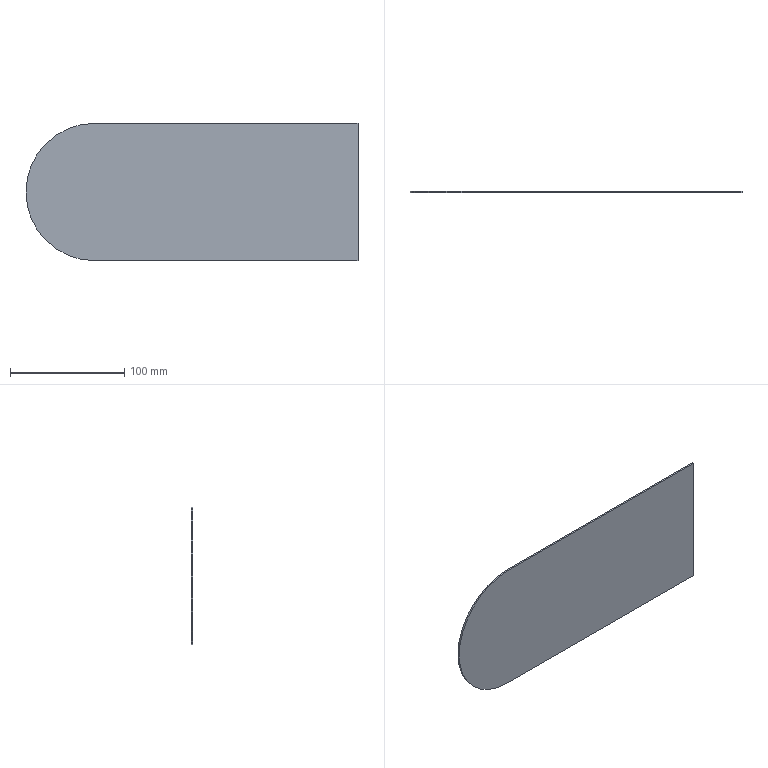Part | SolidWorks | features BaseBody 1 | 1 solid | 6 faces | box 290 x 1.5 x 120 mm | volume 49882 mm3 | plane 5 | cylinder 1 | commonest cylinder face diameters 120 x1
STEP:
#1=CARTESIAN_POINT('',(-115.,-1.5,60.));
#2=VERTEX_POINT('',#1);
#3=CARTESIAN_POINT('',(115.,-1.5,60.));
#4=VERTEX_POINT('',#3);
#5=CARTESIAN_POINT('',(-115.,-1.5,60.));
#6=DIRECTION('',(1.,0.,0.));
#7=VECTOR('',#6,1000.);
#8=LINE('',#5,#7);
#9=EDGE_CURVE('',#2,#4,#8,.T.);
#10=ORIENTED_EDGE('',*,*,#9,.F.);
#11=CARTESIAN_POINT('',(-115.,-1.5,-60.));
#12=VERTEX_POINT('',#11);
#13=CARTESIAN_POINT('',(-115.,-1.5,0.));
#14=DIRECTION('',(0.,1.,0.));
#15=DIRECTION('',(0.,0.,1.));
#16=AXIS2_PLACEMENT_3D('',#13,#14,#15);
#17=CIRCLE('',#16,60.);
#18=EDGE_CURVE('',#12,#2,#17,.T.);
#19=ORIENTED_EDGE('',*,*,#18,.F.);
#20=CARTESIAN_POINT('',(115.,-1.5,-60.));
#21=VERTEX_POINT('',#20);
#22=CARTESIAN_POINT('',(-115.,-1.5,-60.));
#23=DIRECTION('',(-1.,0.,0.));
#24=VECTOR('',#23,1000.);
#25=LINE('',#22,#24);
#26=EDGE_CURVE('',#21,#12,#25,.T.);
#27=ORIENTED_EDGE('',*,*,#26,.F.);
#28=CARTESIAN_POINT('',(115.,-1.5,0.));
#29=DIRECTION('',(0.,0.,-1.));
#30=VECTOR('',#29,1000.);
#31=LINE('',#28,#30);
#32=EDGE_CURVE('',#4,#21,#31,.T.);
#33=ORIENTED_EDGE('',*,*,#32,.F.);
#34=EDGE_LOOP('',(#10,#19,#27,#33));
#35=FACE_OUTER_BOUND('',#34,.T.);
#36=CARTESIAN_POINT('',(-115.,-1.5,0.));
#37=DIRECTION('',(0.,1.,0.));
#38=DIRECTION('',(0.,0.,1.));
#39=AXIS2_PLACEMENT_3D('',#36,#37,#38);
#40=PLANE('',#39);
#41=ADVANCED_FACE('',(#35),#40,.F.);
#42=ORIENTED_EDGE('',*,*,#32,.T.);
#43=CARTESIAN_POINT('',(115.,0.,-60.));
#44=VERTEX_POINT('',#43);
#45=CARTESIAN_POINT('',(115.,-1.5,-60.));
#46=DIRECTION('',(0.,1.,0.));
#47=VECTOR('',#46,1000.);
#48=LINE('',#45,#47);
#49=EDGE_CURVE('',#21,#44,#48,.T.);
#50=ORIENTED_EDGE('',*,*,#49,.T.);
#51=CARTESIAN_POINT('',(115.,0.,60.));
#52=VERTEX_POINT('',#51);
#53=CARTESIAN_POINT('',(115.,0.,60.));
#54=DIRECTION('',(0.,0.,1.));
#55=VECTOR('',#54,1000.);
#56=LINE('',#53,#55);
#57=EDGE_CURVE('',#44,#52,#56,.T.);
#58=ORIENTED_EDGE('',*,*,#57,.T.);
#59=CARTESIAN_POINT('',(115.,-1.5,60.));
#60=DIRECTION('',(0.,-1.,0.));
#61=VECTOR('',#60,1000.);
#62=LINE('',#59,#61);
#63=EDGE_CURVE('',#52,#4,#62,.T.);
#64=ORIENTED_EDGE('',*,*,#63,.T.);
#65=EDGE_LOOP('',(#42,#50,#58,#64));
#66=FACE_OUTER_BOUND('',#65,.T.);
#67=CARTESIAN_POINT('',(115.,-1.5,60.));
#68=DIRECTION('',(1.,0.,0.));
#69=DIRECTION('',(0.,0.,-1.));
#70=AXIS2_PLACEMENT_3D('',#67,#68,#69);
#71=PLANE('',#70);
#72=ADVANCED_FACE('',(#66),#71,.T.);
#73=ORIENTED_EDGE('',*,*,#9,.T.);
#74=ORIENTED_EDGE('',*,*,#63,.F.);
#75=CARTESIAN_POINT('',(-115.,0.,60.));
#76=VERTEX_POINT('',#75);
#77=CARTESIAN_POINT('',(-115.,0.,60.));
#78=DIRECTION('',(-1.,0.,0.));
#79=VECTOR('',#78,1000.);
#80=LINE('',#77,#79);
#81=EDGE_CURVE('',#52,#76,#80,.T.);
#82=ORIENTED_EDGE('',*,*,#81,.T.);
#83=CARTESIAN_POINT('',(-115.,-1.5,60.));
#84=DIRECTION('',(0.,-1.,0.));
#85=VECTOR('',#84,1000.);
#86=LINE('',#83,#85);
#87=EDGE_CURVE('',#76,#2,#86,.T.);
#88=ORIENTED_EDGE('',*,*,#87,.T.);
#89=EDGE_LOOP('',(#73,#74,#82,#88));
#90=FACE_OUTER_BOUND('',#89,.T.);
#91=CARTESIAN_POINT('',(-115.,-1.5,60.));
#92=DIRECTION('',(0.,0.,1.));
#93=DIRECTION('',(1.,0.,0.));
#94=AXIS2_PLACEMENT_3D('',#91,#92,#93);
#95=PLANE('',#94);
#96=ADVANCED_FACE('',(#90),#95,.T.);
#97=ORIENTED_EDGE('',*,*,#18,.T.);
#98=ORIENTED_EDGE('',*,*,#87,.F.);
#99=CARTESIAN_POINT('',(-115.,0.,-60.));
#100=VERTEX_POINT('',#99);
#101=CARTESIAN_POINT('',(-115.,0.,0.));
#102=DIRECTION('',(0.,-1.,0.));
#103=DIRECTION('',(0.,0.,1.));
#104=AXIS2_PLACEMENT_3D('',#101,#102,#103);
#105=CIRCLE('',#104,60.);
#106=EDGE_CURVE('',#76,#100,#105,.T.);
#107=ORIENTED_EDGE('',*,*,#106,.T.);
#108=CARTESIAN_POINT('',(-115.,-1.5,-60.));
#109=DIRECTION('',(0.,-1.,0.));
#110=VECTOR('',#109,1000.);
#111=LINE('',#108,#110);
#112=EDGE_CURVE('',#100,#12,#111,.T.);
#113=ORIENTED_EDGE('',*,*,#112,.T.);
#114=EDGE_LOOP('',(#97,#98,#107,#113));
#115=FACE_OUTER_BOUND('',#114,.T.);
#116=CARTESIAN_POINT('',(-115.,-1.5,0.));
#117=DIRECTION('',(0.,1.,0.));
#118=DIRECTION('',(0.,0.,1.));
#119=AXIS2_PLACEMENT_3D('',#116,#117,#118);
#120=CYLINDRICAL_SURFACE('',#119,60.);
#121=ADVANCED_FACE('',(#115),#120,.T.);
#122=ORIENTED_EDGE('',*,*,#26,.T.);
#123=ORIENTED_EDGE('',*,*,#112,.F.);
#124=CARTESIAN_POINT('',(-115.,0.,-60.));
#125=DIRECTION('',(1.,0.,0.));
#126=VECTOR('',#125,1000.);
#127=LINE('',#124,#126);
#128=EDGE_CURVE('',#100,#44,#127,.T.);
#129=ORIENTED_EDGE('',*,*,#128,.T.);
#130=ORIENTED_EDGE('',*,*,#49,.F.);
#131=EDGE_LOOP('',(#122,#123,#129,#130));
#132=FACE_OUTER_BOUND('',#131,.T.);
#133=CARTESIAN_POINT('',(-115.,-1.5,-60.));
#134=DIRECTION('',(0.,0.,-1.));
#135=DIRECTION('',(-1.,0.,0.));
#136=AXIS2_PLACEMENT_3D('',#133,#134,#135);
#137=PLANE('',#136);
#138=ADVANCED_FACE('',(#132),#137,.T.);
#139=ORIENTED_EDGE('',*,*,#106,.F.);
#140=ORIENTED_EDGE('',*,*,#81,.F.);
#141=ORIENTED_EDGE('',*,*,#57,.F.);
#142=ORIENTED_EDGE('',*,*,#128,.F.);
#143=EDGE_LOOP('',(#139,#140,#141,#142));
#144=FACE_OUTER_BOUND('',#143,.T.);
#145=CARTESIAN_POINT('',(-115.,0.,0.));
#146=DIRECTION('',(0.,1.,0.));
#147=DIRECTION('',(0.,0.,1.));
#148=AXIS2_PLACEMENT_3D('',#145,#146,#147);
#149=PLANE('',#148);
#150=ADVANCED_FACE('',(#144),#149,.T.);
#151=CLOSED_SHELL('',(#41,#72,#96,#121,#138,#150));
#152=MANIFOLD_SOLID_BREP('',#151);
#153=CARTESIAN_POINT('',(0.,0.,0.));
#154=DIRECTION('',(0.,0.,1.));
#155=DIRECTION('',(1.,0.,0.));
#156=AXIS2_PLACEMENT_3D('',#153,#154,#155);
#157=(LENGTH_UNIT()NAMED_UNIT(*)SI_UNIT(.MILLI.,.METRE.));
#158=UNCERTAINTY_MEASURE_WITH_UNIT(LENGTH_MEASURE(0.00001),#157,'','');
#159=(NAMED_UNIT(*)PLANE_ANGLE_UNIT()SI_UNIT($,.RADIAN.));
#160=(NAMED_UNIT(*)SI_UNIT($,.STERADIAN.)SOLID_ANGLE_UNIT());
#161=(GEOMETRIC_REPRESENTATION_CONTEXT(3)GLOBAL_UNCERTAINTY_ASSIGNED_CONTEXT((#158))GLOBAL_UNIT_ASSIGNED_CONTEXT((#157,#159,#160))REPRESENTATION_CONTEXT('',''));
#162=ADVANCED_BREP_SHAPE_REPRESENTATION('',(#152,#156),#161);